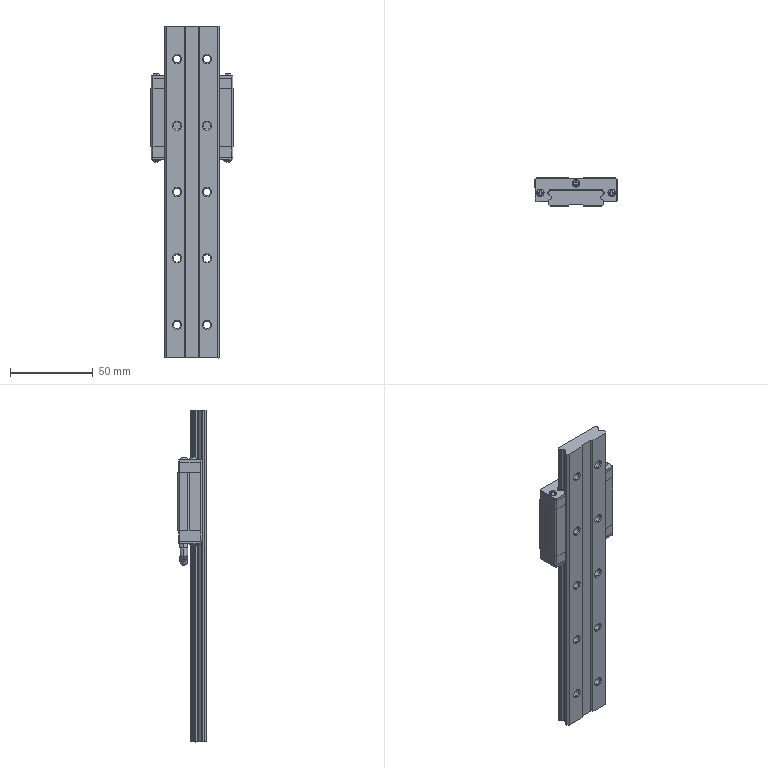Part | SolidWorks | 13 solids | 709 faces | box 50 x 17 x 200 mm | volume 78654 mm3 | plane 347 | cylinder 205 | cone 114 | spline 22 | torus 21 | commonest cylinder face diameters 1 x60 0.77 x36 4.5 x32 3 x26 8 x20 4 x13